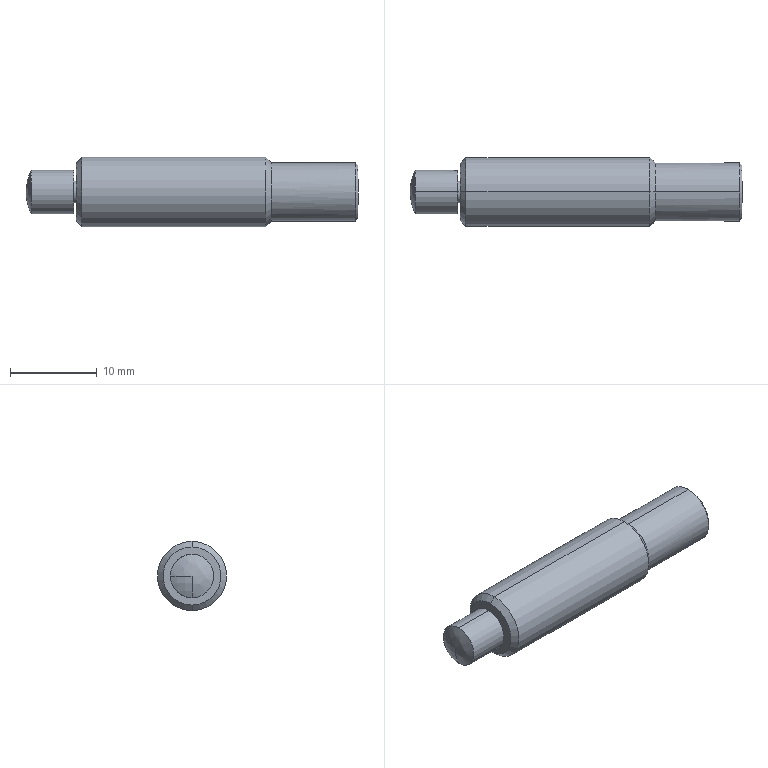Part | STEP file | P649653_YSRT_5_5_C_1 | 1 solid | 27 faces | box 38.3 x 8 x 8 mm | volume 1568 mm3 | plane 10 | cylinder 8 | cone 7 | spline 2 | commonest cylinder face diameters 2.5 x2 5 x2 6.7 x2 8 x2